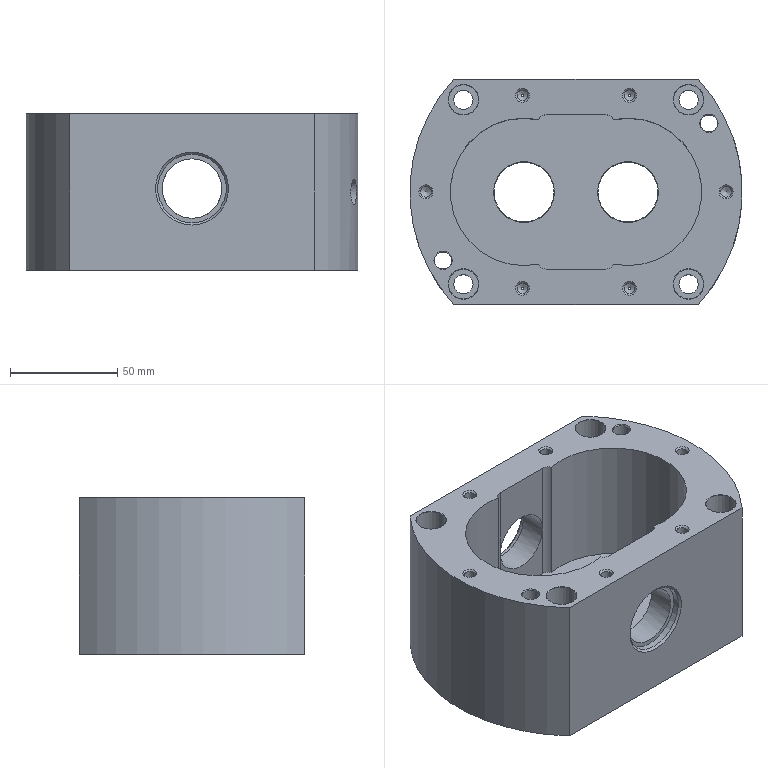NC program | NX | posted with a generic post | part box 155 x 105 x 73.2 mm
Lines 4389 to 5291 of 150882:
(ZLEVEL_PROFILE_COPY , TOOL : D6)
N8734 T06 M6
N8736 G54
N8738 G17 G0 G90 X37.497 Y-43.8 B0. C0. S5000 M3
N8740 G43 Z30. H6
N8742 Z-0.1
N8744 G94 G1 X38.324 Y-44.786 F1000.
N8746 G3 X38.784 Y-45. R0.6
N8748 G1 X41. F1600.
N8750 Y-42.784
N8752 G3 X40.786 Y-42.324 R0.6
N8754 G1 X39.8 Y-41.497
N8756 G0 X37.497 Y-43.8 Z-0.2
N8758 G1 X38.324 Y-44.786 F1000.
N8760 G3 X38.784 Y-45. R0.6
N8762 G1 X41. F1600.
N8764 Y-42.784
N8766 G3 X40.786 Y-42.324 R0.6
N8768 G1 X39.8 Y-41.497
N8770 G0 X37.497 Y-43.8 Z-0.3
N8772 G1 X38.324 Y-44.786 F1000.
N8774 G3 X38.784 Y-45. R0.6
N8776 G1 X41. F1600.
N8778 Y-42.784
N8780 G3 X40.786 Y-42.324 R0.6
N8782 G1 X39.8 Y-41.497
N8784 G0 X37.497 Y-43.8 Z-0.4
N8786 G1 X38.324 Y-44.786 F1000.
N8788 G3 X38.784 Y-45. R0.6
N8790 G1 X41. F1600.
N8792 Y-42.784
N8794 G3 X40.786 Y-42.324 R0.6
N8796 G1 X39.8 Y-41.497
N8798 G0 X37.497 Y-43.8 Z-0.5
N8800 G1 X38.324 Y-44.786 F1000.
N8802 G3 X38.784 Y-45. R0.6
N8804 G1 X41. F1600.
N8806 Y-42.784
N8808 G3 X40.786 Y-42.324 R0.6
N8810 G1 X39.8 Y-41.497
N8812 G0 X37.497 Y-43.8 Z-0.6
N8814 G1 X38.324 Y-44.786 F1000.
N8816 G3 X38.784 Y-45. R0.6
N8818 G1 X41. F1600.
N8820 Y-42.784
N8822 G3 X40.786 Y-42.324 R0.6
N8824 G1 X39.8 Y-41.497
N8826 G0 X37.497 Y-43.8 Z-0.7
N8828 G1 X38.324 Y-44.786 F1000.
N8830 G3 X38.784 Y-45. R0.6
N8832 G1 X41. F1600.
N8834 Y-42.784
N8836 G3 X40.786 Y-42.324 R0.6
N8838 G1 X39.8 Y-41.497
N8840 G0 X37.497 Y-43.8 Z-0.8
N8842 G1 X38.324 Y-44.786 F1000.
N8844 G3 X38.784 Y-45. R0.6
N8846 G1 X41. F1600.
N8848 Y-42.784
N8850 G3 X40.786 Y-42.324 R0.6
N8852 G1 X39.8 Y-41.497
N8854 G0 X37.497 Y-43.8 Z-0.9
N8856 G1 X38.324 Y-44.786 F1000.
N8858 G3 X38.784 Y-45. R0.6
N8860 G1 X41. F1600.
N8862 Y-42.784
N8864 G3 X40.786 Y-42.324 R0.6
N8866 G1 X39.8 Y-41.497
N8868 G0 X37.497 Y-43.8 Z-1.
N8870 G1 X38.324 Y-44.786 F1000.
N8872 G3 X38.784 Y-45. R0.6
N8874 G1 X41. F1600.
N8876 Y-42.784
N8878 G3 X40.786 Y-42.324 R0.6
N8880 G1 X39.8 Y-41.497
N8882 G0 X37.497 Y-43.8 Z-1.1
N8884 G1 X38.324 Y-44.786 F1000.
N8886 G3 X38.784 Y-45. R0.6
N8888 G1 X41. F1600.
N8890 Y-42.784
N8892 G3 X40.786 Y-42.324 R0.6
N8894 G1 X39.8 Y-41.497
N8896 G0 X37.497 Y-43.8 Z-1.2
N8898 G1 X38.324 Y-44.786 F1000.
N8900 G3 X38.784 Y-45. R0.6
N8902 G1 X41. F1600.
N8904 Y-42.784
N8906 G3 X40.786 Y-42.324 R0.6
N8908 G1 X39.8 Y-41.497
N8910 G0 X37.497 Y-43.8 Z-1.3
N8912 G1 X38.324 Y-44.786 F1000.
N8914 G3 X38.784 Y-45. R0.6
N8916 G1 X41. F1600.
N8918 Y-42.784
N8920 G3 X40.786 Y-42.324 R0.6
N8922 G1 X39.8 Y-41.497
N8924 G0 X37.497 Y-43.8 Z-1.4
N8926 G1 X38.324 Y-44.786 F1000.
N8928 G3 X38.784 Y-45. R0.6
N8930 G1 X41. F1600.
N8932 Y-42.784
N8934 G3 X40.786 Y-42.324 R0.6
N8936 G1 X39.8 Y-41.497
N8938 G0 X37.497 Y-43.8 Z-1.5
N8940 G1 X38.324 Y-44.786 F1000.
N8942 G3 X38.784 Y-45. R0.6
N8944 G1 X41. F1600.
N8946 Y-42.784
N8948 G3 X40.786 Y-42.324 R0.6
N8950 G1 X39.8 Y-41.497
N8952 G0 X37.497 Y-43.8 Z-1.6
N8954 G1 X38.324 Y-44.786 F1000.
N8956 G3 X38.784 Y-45. R0.6
N8958 G1 X41. F1600.
N8960 Y-42.784
N8962 G3 X40.786 Y-42.324 R0.6
N8964 G1 X39.8 Y-41.497
N8966 G0 X37.497 Y-43.8 Z-1.7
N8968 G1 X38.324 Y-44.786 F1000.
N8970 G3 X38.784 Y-45. R0.6
N8972 G1 X41. F1600.
N8974 Y-42.784
N8976 G3 X40.786 Y-42.324 R0.6
N8978 G1 X39.8 Y-41.497
N8980 G0 X37.497 Y-43.8 Z-1.8
N8982 G1 X38.324 Y-44.786 F1000.
N8984 G3 X38.784 Y-45. R0.6
N8986 G1 X41. F1600.
N8988 Y-42.784
N8990 G3 X40.786 Y-42.324 R0.6
N8992 G1 X39.8 Y-41.497
N8994 G0 X37.497 Y-43.8 Z-1.9
N8996 G1 X38.324 Y-44.786 F1000.
N8998 G3 X38.784 Y-45. R0.6
N9000 G1 X41. F1600.
N9002 Y-42.784
N9004 G3 X40.786 Y-42.324 R0.6
N9006 G1 X39.8 Y-41.497
N9008 G0 X37.497 Y-43.8 Z-2.
N9010 G1 X38.324 Y-44.786 F1000.
N9012 G3 X38.784 Y-45. R0.6
N9014 G1 X41. F1600.
N9016 Y-42.784
N9018 G3 X40.786 Y-42.324 R0.6
N9020 G1 X39.8 Y-41.497
N9022 G0 X37.497 Y-43.8 Z-2.1
N9024 G1 X38.324 Y-44.786 F1000.
N9026 G3 X38.784 Y-45. R0.6
N9028 G1 X41. F1600.
N9030 Y-42.784
N9032 G3 X40.786 Y-42.324 R0.6
N9034 G1 X39.8 Y-41.497
N9036 G0 X37.497 Y-43.8 Z-2.2
N9038 G1 X38.324 Y-44.786 F1000.
N9040 G3 X38.784 Y-45. R0.6
N9042 G1 X41. F1600.
N9044 Y-42.784
N9046 G3 X40.786 Y-42.324 R0.6
N9048 G1 X39.8 Y-41.497
N9050 G0 X37.497 Y-43.8 Z-2.3
N9052 G1 X38.324 Y-44.786 F1000.
N9054 G3 X38.784 Y-45. R0.6
N9056 G1 X41. F1600.
N9058 Y-42.784
N9060 G3 X40.786 Y-42.324 R0.6
N9062 G1 X39.8 Y-41.497
N9064 G0 X37.497 Y-43.8 Z-2.4
N9066 G1 X38.324 Y-44.786 F1000.
N9068 G3 X38.784 Y-45. R0.6
N9070 G1 X41. F1600.
N9072 Y-42.784
N9074 G3 X40.786 Y-42.324 R0.6
N9076 G1 X39.8 Y-41.497
N9078 G0 X37.497 Y-43.8 Z-2.5
N9080 G1 X38.324 Y-44.786 F1000.
N9082 G3 X38.784 Y-45. R0.6
N9084 G1 X41. F1600.
N9086 Y-42.784
N9088 G3 X40.786 Y-42.324 R0.6
N9090 G1 X39.8 Y-41.497
N9092 G0 X37.497 Y-43.8 Z-2.6
N9094 G1 X38.324 Y-44.786 F1000.
N9096 G3 X38.784 Y-45. R0.6
N9098 G1 X41. F1600.
N9100 Y-42.784
N9102 G3 X40.786 Y-42.324 R0.6
N9104 G1 X39.8 Y-41.497
N9106 G0 X37.497 Y-43.8 Z-2.7
N9108 G1 X38.324 Y-44.786 F1000.
N9110 G3 X38.784 Y-45. R0.6
N9112 G1 X41. F1600.
N9114 Y-42.784
N9116 G3 X40.786 Y-42.324 R0.6
N9118 G1 X39.8 Y-41.497
N9120 G0 X37.497 Y-43.8 Z-2.8
N9122 G1 X38.324 Y-44.786 F1000.
N9124 G3 X38.784 Y-45. R0.6
N9126 G1 X41. F1600.
N9128 Y-42.784
N9130 G3 X40.786 Y-42.324 R0.6
N9132 G1 X39.8 Y-41.497
N9134 G0 X37.497 Y-43.8 Z-2.9
N9136 G1 X38.324 Y-44.786 F1000.
N9138 G3 X38.784 Y-45. R0.6
N9140 G1 X41. F1600.
N9142 Y-42.784
N9144 G3 X40.786 Y-42.324 R0.6
N9146 G1 X39.8 Y-41.497
N9148 G0 X37.497 Y-43.8 Z-3.
N9150 G1 X38.324 Y-44.786 F1000.
N9152 G3 X38.784 Y-45. R0.6
N9154 G1 X41. F1600.
N9156 Y-42.784
N9158 G3 X40.786 Y-42.324 R0.6
N9160 G1 X39.8 Y-41.497
N9162 G0 X37.497 Y-43.8 Z-3.1
N9164 G1 X38.324 Y-44.786 F1000.
N9166 G3 X38.784 Y-45. R0.6
N9168 G1 X41. F1600.
N9170 Y-42.784
N9172 G3 X40.786 Y-42.324 R0.6
N9174 G1 X39.8 Y-41.497
N9176 G0 X37.497 Y-43.8 Z-3.2
N9178 G1 X38.324 Y-44.786 F1000.
N9180 G3 X38.784 Y-45. R0.6
N9182 G1 X41. F1600.
N9184 Y-42.784
N9186 G3 X40.786 Y-42.324 R0.6
N9188 G1 X39.8 Y-41.497
N9190 G0 X37.497 Y-43.8 Z-3.3
N9192 G1 X38.324 Y-44.786 F1000.
N9194 G3 X38.784 Y-45. R0.6
N9196 G1 X41. F1600.
N9198 Y-42.784
N9200 G3 X40.786 Y-42.324 R0.6
N9202 G1 X39.8 Y-41.497
N9204 G0 X37.497 Y-43.8 Z-3.4
N9206 G1 X38.324 Y-44.786 F1000.
N9208 G3 X38.784 Y-45. R0.6
N9210 G1 X41. F1600.
N9212 Y-42.784
N9214 G3 X40.786 Y-42.324 R0.6
N9216 G1 X39.8 Y-41.497
N9218 G0 X37.497 Y-43.8 Z-3.5
N9220 G1 X38.324 Y-44.786 F1000.
N9222 G3 X38.784 Y-45. R0.6
N9224 G1 X41. F1600.
N9226 Y-42.784
N9228 G3 X40.786 Y-42.324 R0.6
N9230 G1 X39.8 Y-41.497
N9232 G0 X37.497 Y-43.8 Z-3.6
N9234 G1 X38.324 Y-44.786 F1000.
N9236 G3 X38.784 Y-45. R0.6
N9238 G1 X41. F1600.
N9240 Y-42.784
N9242 G3 X40.786 Y-42.324 R0.6
N9244 G1 X39.8 Y-41.497
N9246 G0 X37.497 Y-43.8 Z-3.7
N9248 G1 X38.324 Y-44.786 F1000.
N9250 G3 X38.784 Y-45. R0.6
N9252 G1 X41. F1600.
N9254 Y-42.784
N9256 G3 X40.786 Y-42.324 R0.6
N9258 G1 X39.8 Y-41.497
N9260 G0 X37.497 Y-43.8 Z-3.8
N9262 G1 X38.324 Y-44.786 F1000.
N9264 G3 X38.784 Y-45. R0.6
N9266 G1 X41. F1600.
N9268 Y-42.784
N9270 G3 X40.786 Y-42.324 R0.6
N9272 G1 X39.8 Y-41.497
N9274 G0 X37.497 Y-43.8 Z-3.9
N9276 G1 X38.324 Y-44.786 F1000.
N9278 G3 X38.784 Y-45. R0.6
N9280 G1 X41. F1600.
N9282 Y-42.784
N9284 G3 X40.786 Y-42.324 R0.6
N9286 G1 X39.8 Y-41.497
N9288 G0 X37.497 Y-43.8 Z-4.
N9290 G1 X38.324 Y-44.786 F1000.
N9292 G3 X38.784 Y-45. R0.6
N9294 G1 X41. F1600.
N9296 Y-42.784
N9298 G3 X40.786 Y-42.324 R0.6
N9300 G1 X39.8 Y-41.497
N9302 G0 X37.497 Y-43.8 Z-4.1
N9304 G1 X38.324 Y-44.786 F1000.
N9306 G3 X38.784 Y-45. R0.6
N9308 G1 X41. F1600.
N9310 Y-42.784
N9312 G3 X40.786 Y-42.324 R0.6
N9314 G1 X39.8 Y-41.497
N9316 G0 X37.497 Y-43.8 Z-4.2
N9318 G1 X38.324 Y-44.786 F1000.
N9320 G3 X38.784 Y-45. R0.6
N9322 G1 X41. F1600.
N9324 Y-42.784
N9326 G3 X40.786 Y-42.324 R0.6
N9328 G1 X39.8 Y-41.497
N9330 G0 X37.497 Y-43.8 Z-4.3
N9332 G1 X38.324 Y-44.786 F1000.
N9334 G3 X38.784 Y-45. R0.6
N9336 G1 X41. F1600.
N9338 Y-42.784
N9340 G3 X40.786 Y-42.324 R0.6
N9342 G1 X39.8 Y-41.497
N9344 G0 X37.497 Y-43.8 Z-4.4
N9346 G1 X38.324 Y-44.786 F1000.
N9348 G3 X38.784 Y-45. R0.6
N9350 G1 X41. F1600.
N9352 Y-42.784
N9354 G3 X40.786 Y-42.324 R0.6
N9356 G1 X39.8 Y-41.497
N9358 G0 X37.497 Y-43.8 Z-4.5
N9360 G1 X38.324 Y-44.786 F1000.
N9362 G3 X38.784 Y-45. R0.6
N9364 G1 X41. F1600.
N9366 Y-42.784
N9368 G3 X40.786 Y-42.324 R0.6
N9370 G1 X39.8 Y-41.497
N9372 G0 X37.497 Y-43.8 Z-4.6
N9374 G1 X38.324 Y-44.786 F1000.
N9376 G3 X38.784 Y-45. R0.6
N9378 G1 X41. F1600.
N9380 Y-42.784
N9382 G3 X40.786 Y-42.324 R0.6
N9384 G1 X39.8 Y-41.497
N9386 G0 X37.497 Y-43.8 Z-4.7
N9388 G1 X38.324 Y-44.786 F1000.
N9390 G3 X38.784 Y-45. R0.6
N9392 G1 X41. F1600.
N9394 Y-42.784
N9396 G3 X40.786 Y-42.324 R0.6
N9398 G1 X39.8 Y-41.497
N9400 G0 X37.497 Y-43.8 Z-4.8
N9402 G1 X38.324 Y-44.786 F1000.
N9404 G3 X38.784 Y-45. R0.6
N9406 G1 X41. F1600.
N9408 Y-42.784
N9410 G3 X40.786 Y-42.324 R0.6
N9412 G1 X39.8 Y-41.497
N9414 G0 X37.497 Y-43.8 Z-4.9
N9416 G1 X38.324 Y-44.786 F1000.
N9418 G3 X38.784 Y-45. R0.6
N9420 G1 X41. F1600.
N9422 Y-42.784
N9424 G3 X40.786 Y-42.324 R0.6
N9426 G1 X39.8 Y-41.497
N9428 G0 X37.497 Y-43.8 Z-5.
N9430 G1 X38.324 Y-44.786 F1000.
N9432 G3 X38.784 Y-45. R0.6
N9434 G1 X41. F1600.
N9436 Y-42.784
N9438 G3 X40.786 Y-42.324 R0.6
N9440 G1 X39.8 Y-41.497
N9442 G0 X37.497 Y-43.8 Z-5.1
N9444 G1 X38.324 Y-44.786 F1000.
N9446 G3 X38.784 Y-45. R0.6
N9448 G1 X41. F1600.
N9450 Y-42.784
N9452 G3 X40.786 Y-42.324 R0.6
N9454 G1 X39.8 Y-41.497
N9456 G0 X37.497 Y-43.8 Z-5.2
N9458 G1 X38.324 Y-44.786 F1000.
N9460 G3 X38.784 Y-45. R0.6
N9462 G1 X41. F1600.
N9464 Y-42.784
N9466 G3 X40.786 Y-42.324 R0.6
N9468 G1 X39.8 Y-41.497
N9470 G0 X37.497 Y-43.8 Z-5.3
N9472 G1 X38.324 Y-44.786 F1000.
N9474 G3 X38.784 Y-45. R0.6
N9476 G1 X41. F1600.
N9478 Y-42.784
N9480 G3 X40.786 Y-42.324 R0.6
N9482 G1 X39.8 Y-41.497
N9484 G0 X37.497 Y-43.8 Z-5.4
N9486 G1 X38.324 Y-44.786 F1000.
N9488 G3 X38.784 Y-45. R0.6
N9490 G1 X41. F1600.
N9492 Y-42.784
N9494 G3 X40.786 Y-42.324 R0.6
N9496 G1 X39.8 Y-41.497
N9498 G0 X37.497 Y-43.8 Z-5.5
N9500 G1 X38.324 Y-44.786 F1000.
N9502 G3 X38.784 Y-45. R0.6
N9504 G1 X41. F1600.
N9506 Y-42.784
N9508 G3 X40.786 Y-42.324 R0.6
N9510 G1 X39.8 Y-41.497
N9512 G0 X37.497 Y-43.8 Z-5.6
N9514 G1 X38.324 Y-44.786 F1000.
N9516 G3 X38.784 Y-45. R0.6
N9518 G1 X41. F1600.
N9520 Y-42.784
N9522 G3 X40.786 Y-42.324 R0.6
N9524 G1 X39.8 Y-41.497
N9526 G0 X37.497 Y-43.8 Z-5.7
N9528 G1 X38.324 Y-44.786 F1000.
N9530 G3 X38.784 Y-45. R0.6
N9532 G1 X41. F1600.
N9534 Y-42.784
N9536 G3 X40.786 Y-42.324 R0.6
N9538 G1 X39.8 Y-41.497
N9540 G0 X37.497 Y-43.8 Z-5.8
N9542 G1 X38.324 Y-44.786 F1000.
N9544 G3 X38.784 Y-45. R0.6
N9546 G1 X41. F1600.
N9548 Y-42.784
N9550 G3 X40.786 Y-42.324 R0.6
N9552 G1 X39.8 Y-41.497
N9554 G0 X37.497 Y-43.8 Z-5.9
N9556 G1 X38.324 Y-44.786 F1000.
N9558 G3 X38.784 Y-45. R0.6
N9560 G1 X41. F1600.
N9562 Y-42.784
N9564 G3 X40.786 Y-42.324 R0.6
N9566 G1 X39.8 Y-41.497
N9568 G0 X37.497 Y-43.8 Z-6.
N9570 G1 X38.324 Y-44.786 F1000.
N9572 G3 X38.784 Y-45. R0.6
N9574 G1 X41. F1600.
N9576 Y-42.784
N9578 G3 X40.786 Y-42.324 R0.6
N9580 G1 X39.8 Y-41.497
N9582 G0 X37.497 Y-43.8 Z-6.1
N9584 G1 X38.324 Y-44.786 F1000.
N9586 G3 X38.784 Y-45. R0.6
N9588 G1 X41. F1600.
N9590 Y-42.784
N9592 G3 X40.786 Y-42.324 R0.6
N9594 G1 X39.8 Y-41.497
N9596 G0 X37.497 Y-43.8 Z-6.2
N9598 G1 X38.324 Y-44.786 F1000.
N9600 G3 X38.784 Y-45. R0.6
N9602 G1 X41. F1600.
N9604 Y-42.784
N9606 G3 X40.786 Y-42.324 R0.6
N9608 G1 X39.8 Y-41.497
N9610 G0 X37.497 Y-43.8 Z-6.3
N9612 G1 X38.324 Y-44.786 F1000.
N9614 G3 X38.784 Y-45. R0.6
N9616 G1 X41. F1600.
N9618 Y-42.784
N9620 G3 X40.786 Y-42.324 R0.6
N9622 G1 X39.8 Y-41.497
N9624 G0 X37.497 Y-43.8 Z-6.4
N9626 G1 X38.324 Y-44.786 F1000.
N9628 G3 X38.784 Y-45. R0.6
N9630 G1 X41. F1600.
N9632 Y-42.784
N9634 G3 X40.786 Y-42.324 R0.6
N9636 G1 X39.8 Y-41.497
N9638 G0 X37.497 Y-43.8 Z-6.5
N9640 G1 X38.324 Y-44.786 F1000.
N9642 G3 X38.784 Y-45. R0.6
N9644 G1 X41. F1600.
N9646 Y-42.784
N9648 G3 X40.786 Y-42.324 R0.6
N9650 G1 X39.8 Y-41.497
N9652 G0 X37.497 Y-43.8 Z-6.6
N9654 G1 X38.324 Y-44.786 F1000.
N9656 G3 X38.784 Y-45. R0.6
N9658 G1 X41. F1600.
N9660 Y-42.784
N9662 G3 X40.786 Y-42.324 R0.6
N9664 G1 X39.8 Y-41.497
N9666 G0 X37.497 Y-43.8 Z-6.7
N9668 G1 X38.324 Y-44.786 F1000.
N9670 G3 X38.784 Y-45. R0.6
N9672 G1 X41. F1600.
N9674 Y-42.784
N9676 G3 X40.786 Y-42.324 R0.6
N9678 G1 X39.8 Y-41.497
N9680 G0 X37.497 Y-43.8 Z-6.8
N9682 G1 X38.324 Y-44.786 F1000.
N9684 G3 X38.784 Y-45. R0.6
N9686 G1 X41. F1600.
N9688 Y-42.784
N9690 G3 X40.786 Y-42.324 R0.6
N9692 G1 X39.8 Y-41.497
N9694 G0 X37.497 Y-43.8 Z-6.9
N9696 G1 X38.324 Y-44.786 F1000.
N9698 G3 X38.784 Y-45. R0.6
N9700 G1 X41. F1600.
N9702 Y-42.784
N9704 G3 X40.786 Y-42.324 R0.6
N9706 G1 X39.8 Y-41.497
N9708 G0 X37.497 Y-43.8 Z-7.
N9710 G1 X38.324 Y-44.786 F1000.
N9712 G3 X38.784 Y-45. R0.6
N9714 G1 X41. F1600.
N9716 Y-42.784
N9718 G3 X40.786 Y-42.324 R0.6
N9720 G1 X39.8 Y-41.497
N9722 G0 Z30.
N9724 X39.231 Y-36.841
N9726 Z-2.1
N9728 G1 X40.272 Y-36.341 F1000.
N9730 G3 X40.593 Y-35.949 R0.6
N9732 G2 X43.35 Y-32.271 R6. F1600.
N9734 G3 X53.648 Y-23.281 R37.5
N9736 G2 X57.664 Y-21.045 R6.
N9738 G3 X58.096 Y-20.779 R0.6
N9740 G1 X58.732 Y-19.815
N9742 G0 Z30.
N9744 X39.231 Y-36.841
N9746 Z-2.2
N9748 G1 X40.272 Y-36.341 F1000.
N9750 G3 X40.593 Y-35.949 R0.6
N9752 G2 X43.35 Y-32.271 R6. F1600.
N9754 G3 X53.648 Y-23.281 R37.5
N9756 G2 X57.664 Y-21.045 R6.
N9758 G3 X58.096 Y-20.779 R0.6
N9760 G1 X58.732 Y-19.815
N9762 G0 Z30.
N9764 X39.231 Y-36.841
N9766 Z-2.3
N9768 G1 X40.272 Y-36.341 F1000.
N9770 G3 X40.593 Y-35.949 R0.6
N9772 G2 X43.35 Y-32.271 R6. F1600.
N9774 G3 X53.648 Y-23.281 R37.5
N9776 G2 X57.664 Y-21.045 R6.
N9778 G3 X58.096 Y-20.779 R0.6
N9780 G1 X58.732 Y-19.815
N9782 G0 Z30.
N9784 X39.231 Y-36.841
N9786 Z-2.4
N9788 G1 X40.272 Y-36.341 F1000.
N9790 G3 X40.593 Y-35.949 R0.6
N9792 G2 X43.35 Y-32.271 R6. F1600.
N9794 G3 X53.648 Y-23.281 R37.5
N9796 G2 X57.664 Y-21.045 R6.
N9798 G3 X58.096 Y-20.779 R0.6
N9800 G1 X58.732 Y-19.815
N9802 G0 Z30.
N9804 X39.231 Y-36.841
N9806 Z-2.5
N9808 G1 X40.272 Y-36.341 F1000.
N9810 G3 X40.593 Y-35.949 R0.6
N9812 G2 X43.35 Y-32.271 R6. F1600.
N9814 G3 X53.648 Y-23.281 R37.5
N9816 G2 X57.664 Y-21.045 R6.
N9818 G3 X58.096 Y-20.779 R0.6
N9820 G1 X58.732 Y-19.815
N9822 G0 Z30.
N9824 X39.231 Y-36.841
N9826 Z-2.6
N9828 G1 X40.272 Y-36.341 F1000.
N9830 G3 X40.593 Y-35.949 R0.6
N9832 G2 X43.35 Y-32.271 R6. F1600.
N9834 G3 X53.648 Y-23.281 R37.5
N9836 G2 X57.664 Y-21.045 R6.
N9838 G3 X58.096 Y-20.779 R0.6
N9840 G1 X58.732 Y-19.815
N9842 G0 Z30.
N9844 X39.231 Y-36.841
N9846 Z-2.7
N9848 G1 X40.272 Y-36.341 F1000.
N9850 G3 X40.593 Y-35.949 R0.6
N9852 G2 X43.35 Y-32.271 R6. F1600.
N9854 G3 X53.648 Y-23.281 R37.5
N9856 G2 X57.664 Y-21.045 R6.
N9858 G3 X58.096 Y-20.779 R0.6
N9860 G1 X58.732 Y-19.815
N9862 G0 Z30.
N9864 X39.231 Y-36.841
N9866 Z-2.8
N9868 G1 X40.272 Y-36.341 F1000.
N9870 G3 X40.593 Y-35.949 R0.6
N9872 G2 X43.35 Y-32.271 R6. F1600.
N9874 G3 X53.648 Y-23.281 R37.5
N9876 G2 X57.664 Y-21.045 R6.
N9878 G3 X58.096 Y-20.779 R0.6
N9880 G1 X58.732 Y-19.815
N9882 G0 Z30.
N9884 X39.231 Y-36.841
N9886 Z-2.9
N9888 G1 X40.272 Y-36.341 F1000.
N9890 G3 X40.593 Y-35.949 R0.6
N9892 G2 X43.35 Y-32.271 R6. F1600.
N9894 G3 X53.648 Y-23.281 R37.5
N9896 G2 X57.664 Y-21.045 R6.
N9898 G3 X58.096 Y-20.779 R0.6
N9900 G1 X58.732 Y-19.815
N9902 G0 Z30.
N9904 X39.231 Y-36.841
N9906 Z-3.
N9908 G1 X40.272 Y-36.341 F1000.
N9910 G3 X40.593 Y-35.949 R0.6
N9912 G2 X43.35 Y-32.271 R6. F1600.
N9914 G3 X53.648 Y-23.281 R37.5
N9916 G2 X57.664 Y-21.045 R6.
N9918 G3 X58.096 Y-20.779 R0.6
N9920 G1 X58.732 Y-19.815
N9922 G0 Z30.
N9924 X39.231 Y-36.841
N9926 Z-3.1
N9928 G1 X40.272 Y-36.341 F1000.
N9930 G3 X40.593 Y-35.949 R0.6
N9932 G2 X43.35 Y-32.271 R6. F1600.
N9934 G3 X53.648 Y-23.281 R37.5
N9936 G2 X57.664 Y-21.045 R6.
N9938 G3 X58.096 Y-20.779 R0.6
N9940 G1 X58.732 Y-19.815
N9942 G0 Z30.
N9944 X39.231 Y-36.841
N9946 Z-3.2
N9948 G1 X40.272 Y-36.341 F1000.
N9950 G3 X40.593 Y-35.949 R0.6
N9952 G2 X43.35 Y-32.271 R6. F1600.
N9954 G3 X53.648 Y-23.281 R37.5
N9956 G2 X57.664 Y-21.045 R6.
N9958 G3 X58.096 Y-20.779 R0.6
N9960 G1 X58.732 Y-19.815
N9962 G0 Z30.
N9964 X39.231 Y-36.841
N9966 Z-3.3
N9968 G1 X40.272 Y-36.341 F1000.
N9970 G3 X40.593 Y-35.949 R0.6
N9972 G2 X43.35 Y-32.271 R6. F1600.
N9974 G3 X53.648 Y-23.281 R37.5
N9976 G2 X57.664 Y-21.045 R6.
N9978 G3 X58.096 Y-20.779 R0.6
N9980 G1 X58.732 Y-19.815
N9982 G0 Z30.
N9984 X39.231 Y-36.841
N9986 Z-3.4
N9988 G1 X40.272 Y-36.341 F1000.
N9990 G3 X40.593 Y-35.949 R0.6
N9992 G2 X43.35 Y-32.271 R6. F1600.
N9994 G3 X53.648 Y-23.281 R37.5
N9996 G2 X57.664 Y-21.045 R6.
N9998 G3 X58.096 Y-20.779 R0.6
N10000 G1 X58.732 Y-19.815
N10002 G0 Z30.
N10004 X39.231 Y-36.841
N10006 Z-3.5
N10008 G1 X40.272 Y-36.341 F1000.
N10010 G3 X40.593 Y-35.949 R0.6
N10012 G2 X43.35 Y-32.271 R6. F1600.
N10014 G3 X53.648 Y-23.281 R37.5
N10016 G2 X57.664 Y-21.045 R6.
N10018 G3 X58.096 Y-20.779 R0.6
N10020 G1 X58.732 Y-19.815
N10022 G0 Z30.
N10024 X39.231 Y-36.841
N10026 Z-3.6
N10028 G1 X40.272 Y-36.341 F1000.
N10030 G3 X40.593 Y-35.949 R0.6
N10032 G2 X43.35 Y-32.271 R6. F1600.
N10034 G3 X53.648 Y-23.281 R37.5
N10036 G2 X57.664 Y-21.045 R6.
N10038 G3 X58.096 Y-20.779 R0.6
N10040 G1 X58.732 Y-19.815
N10042 G0 Z30.
N10044 X39.231 Y-36.841
N10046 Z-3.7
N10048 G1 X40.272 Y-36.341 F1000.
N10050 G3 X40.593 Y-35.949 R0.6
N10052 G2 X43.35 Y-32.271 R6. F1600.
N10054 G3 X53.648 Y-23.281 R37.5
N10056 G2 X57.664 Y-21.045 R6.
N10058 G3 X58.096 Y-20.779 R0.6
N10060 G1 X58.732 Y-19.815
N10062 G0 Z30.
N10064 X39.231 Y-36.841
N10066 Z-3.8
N10068 G1 X40.272 Y-36.341 F1000.
N10070 G3 X40.593 Y-35.949 R0.6
N10072 G2 X43.35 Y-32.271 R6. F1600.
N10074 G3 X53.648 Y-23.281 R37.5
N10076 G2 X57.664 Y-21.045 R6.
N10078 G3 X58.096 Y-20.779 R0.6
N10080 G1 X58.732 Y-19.815
N10082 G0 Z30.
N10084 X39.231 Y-36.841
N10086 Z-3.9
N10088 G1 X40.272 Y-36.341 F1000.
N10090 G3 X40.593 Y-35.949 R0.6
N10092 G2 X43.35 Y-32.271 R6. F1600.
N10094 G3 X53.648 Y-23.281 R37.5
N10096 G2 X57.664 Y-21.045 R6.
N10098 G3 X58.096 Y-20.779 R0.6
N10100 G1 X58.732 Y-19.815
N10102 G0 Z30.
N10104 X39.231 Y-36.841
N10106 Z-4.
N10108 G1 X40.272 Y-36.341 F1000.
N10110 G3 X40.593 Y-35.949 R0.6
N10112 G2 X43.35 Y-32.271 R6. F1600.
N10114 G3 X53.648 Y-23.281 R37.5
N10116 G2 X57.664 Y-21.045 R6.
N10118 G3 X58.096 Y-20.779 R0.6
N10120 G1 X58.732 Y-19.815
N10122 G0 Z30.
N10124 X39.231 Y-36.841
N10126 Z-4.1
N10128 G1 X40.272 Y-36.341 F1000.
N10130 G3 X40.593 Y-35.949 R0.6
N10132 G2 X43.35 Y-32.271 R6. F1600.
N10134 G3 X53.648 Y-23.281 R37.5
N10136 G2 X57.664 Y-21.045 R6.
N10138 G3 X58.096 Y-20.779 R0.6
N10140 G1 X58.732 Y-19.815
N10142 G0 Z30.
N10144 X39.231 Y-36.841
N10146 Z-4.2
N10148 G1 X40.272 Y-36.341 F1000.
N10150 G3 X40.593 Y-35.949 R0.6
N10152 G2 X43.35 Y-32.271 R6. F1600.
N10154 G3 X53.648 Y-23.281 R37.5
N10156 G2 X57.664 Y-21.045 R6.
N10158 G3 X58.096 Y-20.779 R0.6
N10160 G1 X58.732 Y-19.815
N10162 G0 Z30.
N10164 X39.231 Y-36.841
N10166 Z-4.3
N10168 G1 X40.272 Y-36.341 F1000.
N10170 G3 X40.593 Y-35.949 R0.6
N10172 G2 X43.35 Y-32.271 R6. F1600.
N10174 G3 X53.648 Y-23.281 R37.5
N10176 G2 X57.664 Y-21.045 R6.
N10178 G3 X58.096 Y-20.779 R0.6
N10180 G1 X58.732 Y-19.815
N10182 G0 Z30.
N10184 X39.231 Y-36.841
N10186 Z-4.4
N10188 G1 X40.272 Y-36.341 F1000.
N10190 G3 X40.593 Y-35.949 R0.6
N10192 G2 X43.35 Y-32.271 R6. F1600.
N10194 G3 X53.648 Y-23.281 R37.5
N10196 G2 X57.664 Y-21.045 R6.
N10198 G3 X58.096 Y-20.779 R0.6
N10200 G1 X58.732 Y-19.815
N10202 G0 Z30.
N10204 X39.231 Y-36.841
N10206 Z-4.5
N10208 G1 X40.272 Y-36.341 F1000.
N10210 G3 X40.593 Y-35.949 R0.6
N10212 G2 X43.35 Y-32.271 R6. F1600.
N10214 G3 X53.648 Y-23.281 R37.5
N10216 G2 X57.664 Y-21.045 R6.
N10218 G3 X58.096 Y-20.779 R0.6
N10220 G1 X58.732 Y-19.815
N10222 G0 Z30.
N10224 X39.231 Y-36.841
N10226 Z-4.6
N10228 G1 X40.272 Y-36.341 F1000.
N10230 G3 X40.593 Y-35.949 R0.6
N10232 G2 X43.35 Y-32.271 R6. F1600.
N10234 G3 X53.648 Y-23.281 R37.5
N10236 G2 X57.664 Y-21.045 R6.
N10238 G3 X58.096 Y-20.779 R0.6
N10240 G1 X58.732 Y-19.815
N10242 G0 Z30.
N10244 X39.231 Y-36.841
N10246 Z-4.7
N10248 G1 X40.272 Y-36.341 F1000.
N10250 G3 X40.593 Y-35.949 R0.6
N10252 G2 X43.35 Y-32.271 R6. F1600.
N10254 G3 X53.648 Y-23.281 R37.5
N10256 G2 X57.664 Y-21.045 R6.
N10258 G3 X58.096 Y-20.779 R0.6
N10260 G1 X58.732 Y-19.815
N10262 G0 Z30.
N10264 X39.231 Y-36.841
N10266 Z-4.8
N10268 G1 X40.272 Y-36.341 F1000.
N10270 G3 X40.593 Y-35.949 R0.6
N10272 G2 X43.35 Y-32.271 R6. F1600.
N10274 G3 X53.648 Y-23.281 R37.5
N10276 G2 X57.664 Y-21.045 R6.
N10278 G3 X58.096 Y-20.779 R0.6
N10280 G1 X58.732 Y-19.815
N10282 G0 Z30.
N10284 X39.231 Y-36.841
N10286 Z-4.9
N10288 G1 X40.272 Y-36.341 F1000.
N10290 G3 X40.593 Y-35.949 R0.6
N10292 G2 X43.35 Y-32.271 R6. F1600.
N10294 G3 X53.648 Y-23.281 R37.5
N10296 G2 X57.664 Y-21.045 R6.
N10298 G3 X58.096 Y-20.779 R0.6
N10300 G1 X58.732 Y-19.815
N10302 G0 Z30.
N10304 X39.231 Y-36.841
N10306 Z-5.
N10308 G1 X40.272 Y-36.341 F1000.
N10310 G3 X40.593 Y-35.949 R0.6
N10312 G2 X43.35 Y-32.271 R6. F1600.
N10314 G3 X53.648 Y-23.281 R37.5
N10316 G2 X57.664 Y-21.045 R6.
N10318 G3 X58.096 Y-20.779 R0.6
N10320 G1 X58.732 Y-19.815
N10322 G0 Z30.
N10324 X39.231 Y-36.841
N10326 Z-5.1
N10328 G1 X40.272 Y-36.341 F1000.
N10330 G3 X40.593 Y-35.949 R0.6
N10332 G2 X43.35 Y-32.271 R6. F1600.
N10334 G3 X53.648 Y-23.281 R37.5
N10336 G2 X57.664 Y-21.045 R6.
N10338 G3 X58.096 Y-20.779 R0.6
N10340 G1 X58.732 Y-19.815
N10342 G0 Z30.
N10344 X39.231 Y-36.841
N10346 Z-5.2
N10348 G1 X40.272 Y-36.341 F1000.
N10350 G3 X40.593 Y-35.949 R0.6
N10352 G2 X43.35 Y-32.271 R6. F1600.
N10354 G3 X53.648 Y-23.281 R37.5
N10356 G2 X57.664 Y-21.045 R6.
N10358 G3 X58.096 Y-20.779 R0.6
N10360 G1 X58.732 Y-19.815
N10362 G0 Z30.
N10364 X39.231 Y-36.841
N10366 Z-5.3
N10368 G1 X40.272 Y-36.341 F1000.
N10370 G3 X40.593 Y-35.949 R0.6
N10372 G2 X43.35 Y-32.271 R6. F1600.
N10374 G3 X53.648 Y-23.281 R37.5
N10376 G2 X57.664 Y-21.045 R6.
N10378 G3 X58.096 Y-20.779 R0.6
N10380 G1 X58.732 Y-19.815
N10382 G0 Z30.
N10384 X39.231 Y-36.841
N10386 Z-5.4
N10388 G1 X40.272 Y-36.341 F1000.
N10390 G3 X40.593 Y-35.949 R0.6
N10392 G2 X43.35 Y-32.271 R6. F1600.
N10394 G3 X53.648 Y-23.281 R37.5
N10396 G2 X57.664 Y-21.045 R6.
N10398 G3 X58.096 Y-20.779 R0.6
N10400 G1 X58.732 Y-19.815
N10402 G0 Z30.
N10404 X39.231 Y-36.841
N10406 Z-5.5
N10408 G1 X40.272 Y-36.341 F1000.
N10410 G3 X40.593 Y-35.949 R0.6
N10412 G2 X43.35 Y-32.271 R6. F1600.
N10414 G3 X53.648 Y-23.281 R37.5
N10416 G2 X57.664 Y-21.045 R6.
N10418 G3 X58.096 Y-20.779 R0.6
N10420 G1 X58.732 Y-19.815
N10422 G0 Z30.
N10424 X39.231 Y-36.841
N10426 Z-5.6
N10428 G1 X40.272 Y-36.341 F1000.
N10430 G3 X40.593 Y-35.949 R0.6
N10432 G2 X43.35 Y-32.271 R6. F1600.
N10434 G3 X53.648 Y-23.281 R37.5
N10436 G2 X57.664 Y-21.045 R6.
N10438 G3 X58.096 Y-20.779 R0.6
N10440 G1 X58.732 Y-19.815
N10442 G0 Z30.
N10444 X39.231 Y-36.841
N10446 Z-5.7
N10448 G1 X40.272 Y-36.341 F1000.
N10450 G3 X40.593 Y-35.949 R0.6
N10452 G2 X43.35 Y-32.271 R6. F1600.
N10454 G3 X53.648 Y-23.281 R37.5
N10456 G2 X57.664 Y-21.045 R6.
N10458 G3 X58.096 Y-20.779 R0.6
N10460 G1 X58.732 Y-19.815
N10462 G0 Z30.
N10464 X39.231 Y-36.841
N10466 Z-5.8
N10468 G1 X40.272 Y-36.341 F1000.
N10470 G3 X40.593 Y-35.949 R0.6
N10472 G2 X43.35 Y-32.271 R6. F1600.
N10474 G3 X53.648 Y-23.281 R37.5
N10476 G2 X57.664 Y-21.045 R6.
N10478 G3 X58.096 Y-20.779 R0.6
N10480 G1 X58.732 Y-19.815
N10482 G0 Z30.
N10484 X39.231 Y-36.841
N10486 Z-5.9
N10488 G1 X40.272 Y-36.341 F1000.
N10490 G3 X40.593 Y-35.949 R0.6
N10492 G2 X43.35 Y-32.271 R6. F1600.
N10494 G3 X53.648 Y-23.281 R37.5
N10496 G2 X57.664 Y-21.045 R6.
N10498 G3 X58.096 Y-20.779 R0.6
N10500 G1 X58.732 Y-19.815
N10502 G0 Z30.
N10504 X39.231 Y-36.841
N10506 Z-6.
N10508 G1 X40.272 Y-36.341 F1000.
N10510 G3 X40.593 Y-35.949 R0.6
N10512 G2 X43.35 Y-32.271 R6. F1600.
N10514 G3 X53.648 Y-23.281 R37.5
N10516 G2 X57.664 Y-21.045 R6.
N10518 G3 X58.096 Y-20.779 R0.6
N10520 G1 X58.732 Y-19.815
N10522 G0 Z30.
N10524 X39.231 Y-36.841
N10526 Z-6.1
N10528 G1 X40.272 Y-36.341 F1000.
N10530 G3 X40.593 Y-35.949 R0.6
N10532 G2 X43.35 Y-32.271 R6. F1600.